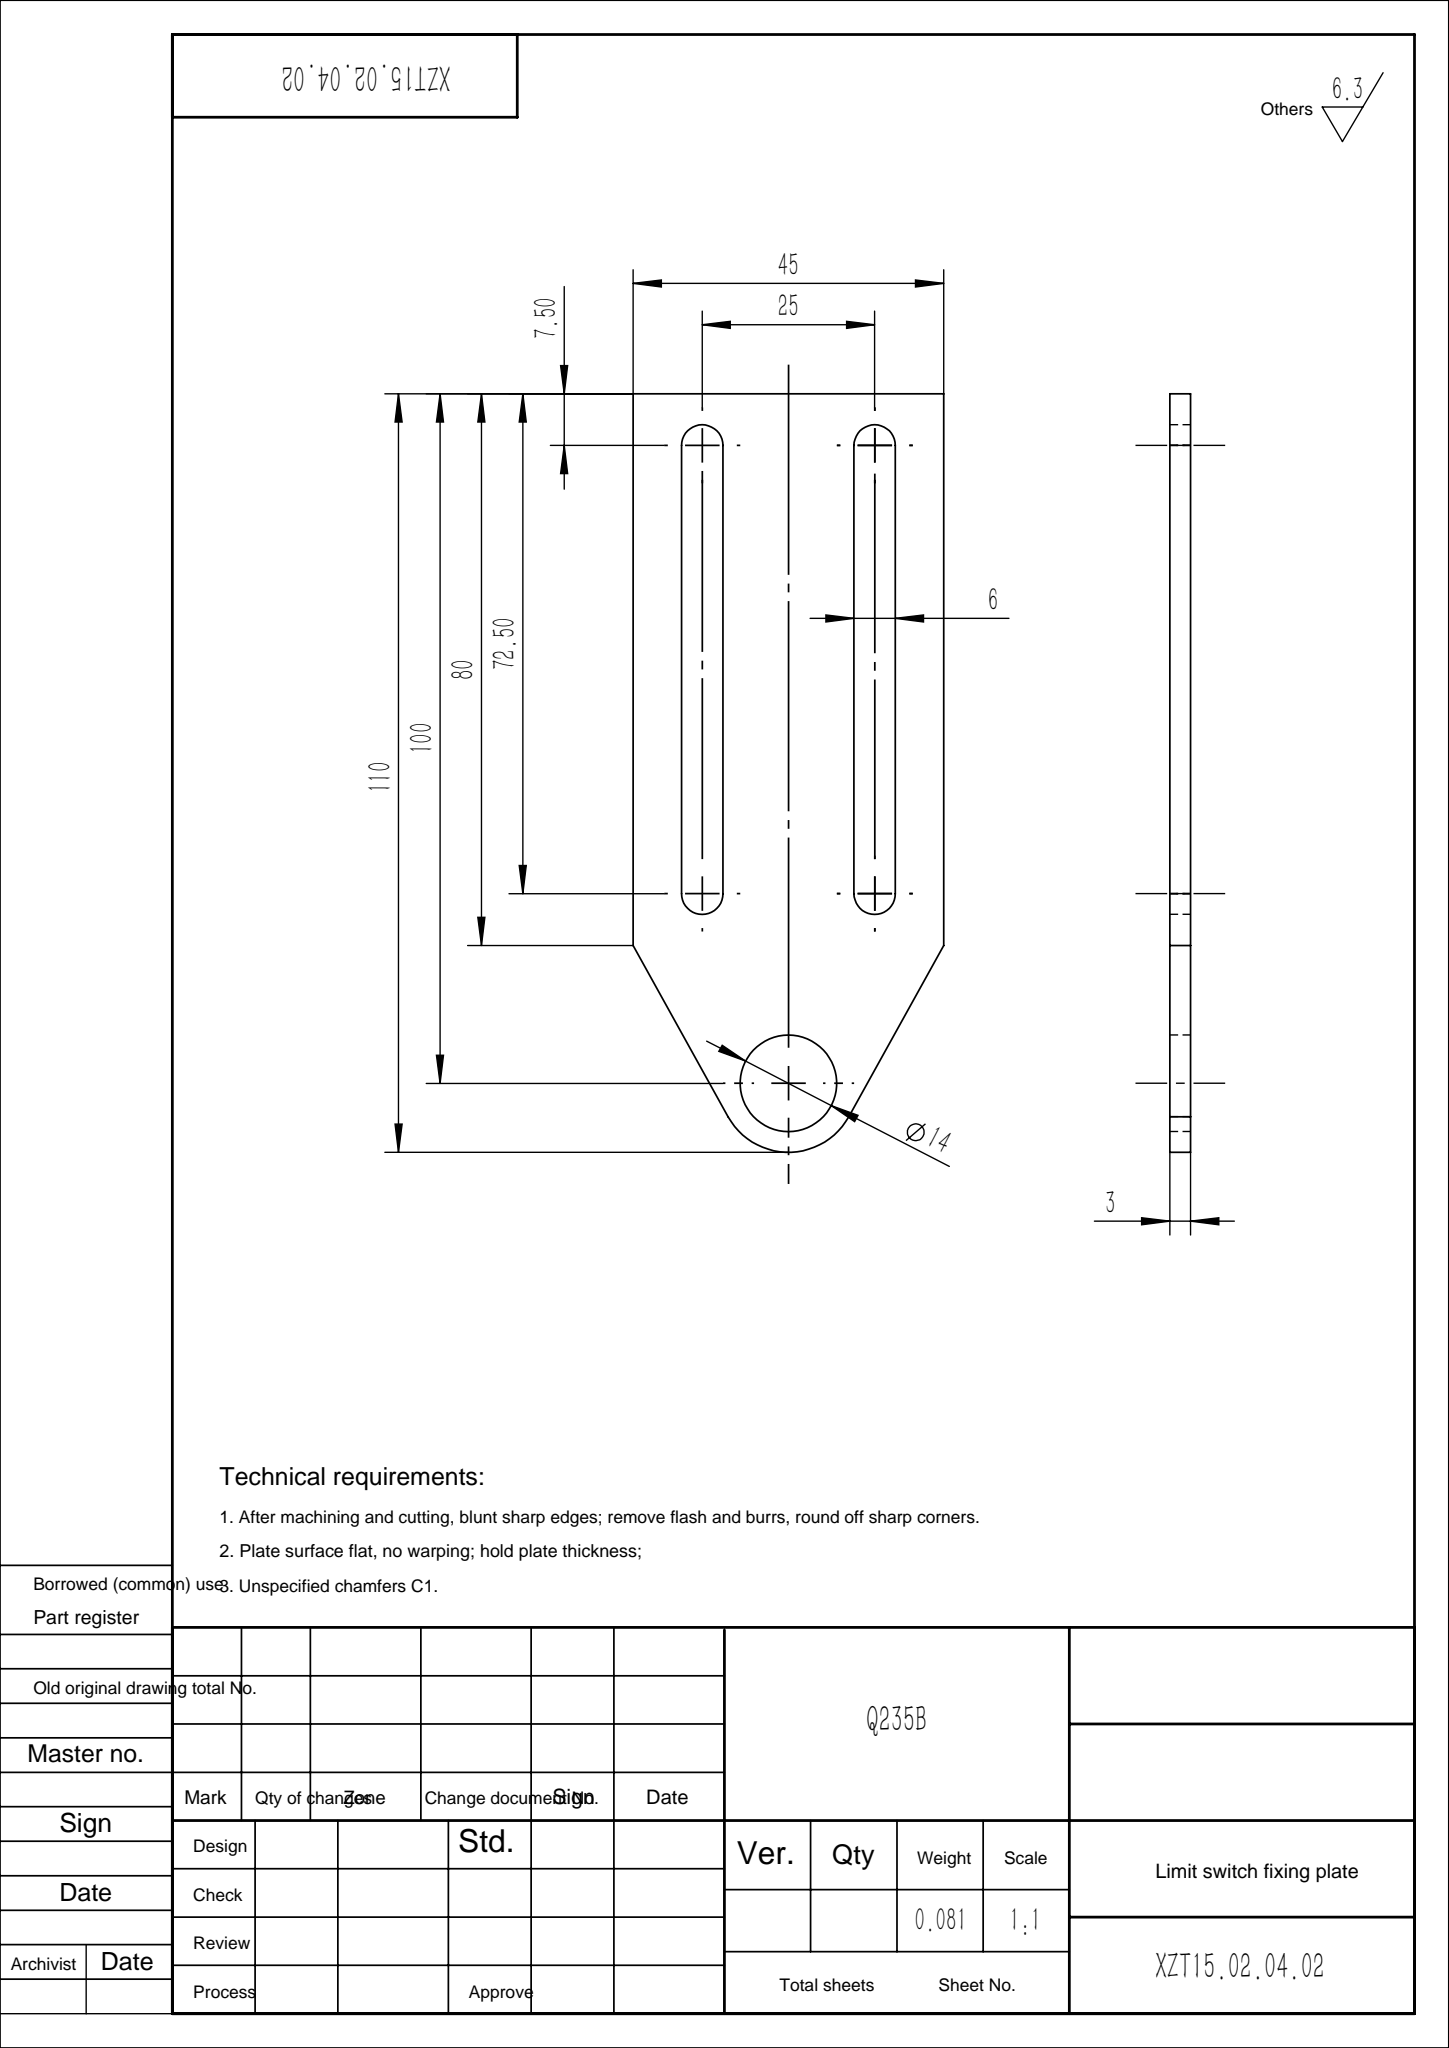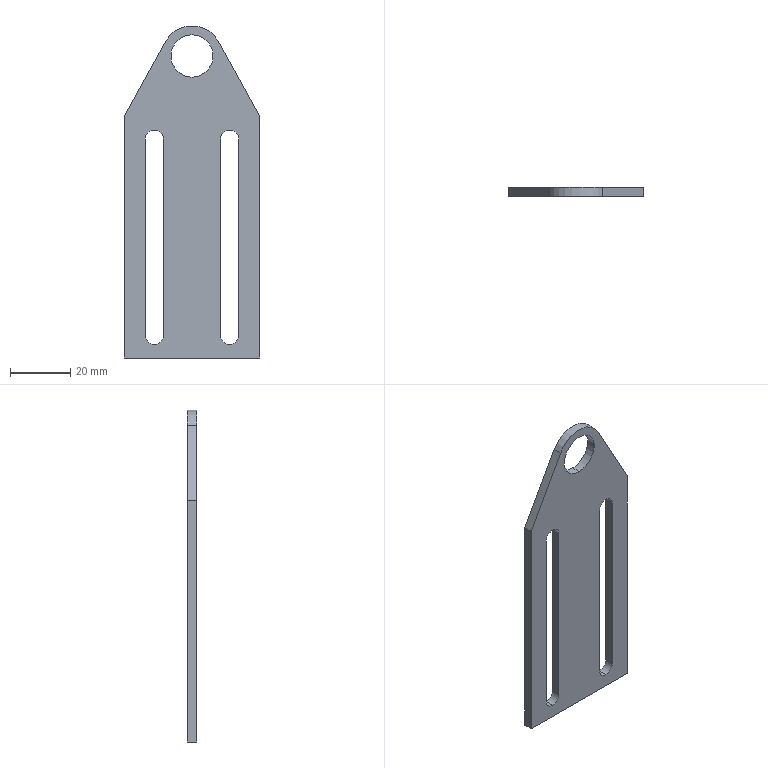Part | SolidWorks | features Extrusion 1 | 1 solid | 20 faces | box 45 x 3 x 110 mm | volume 10350 mm3 | plane 11 | cylinder 9 | commonest cylinder face diameters 6 x6 14 x2 20 x1
STEP:
#1=CARTESIAN_POINT('',(15.5,3.,-92.5));
#2=VERTEX_POINT('',#1);
#3=CARTESIAN_POINT('',(12.5,3.,-95.5));
#4=VERTEX_POINT('',#3);
#5=CARTESIAN_POINT('',(12.5,3.,-92.5));
#6=DIRECTION('',(0.,1.,0.));
#7=DIRECTION('',(0.,0.,-1.));
#8=AXIS2_PLACEMENT_3D('',#5,#6,#7);
#9=CIRCLE('',#8,3.);
#10=EDGE_CURVE('',#2,#4,#9,.T.);
#11=ORIENTED_EDGE('',*,*,#10,.T.);
#12=CARTESIAN_POINT('',(12.5,0.,-95.5));
#13=VERTEX_POINT('',#12);
#14=CARTESIAN_POINT('',(12.5,3.,-95.5));
#15=DIRECTION('',(0.,-1.,0.));
#16=VECTOR('',#15,1000.);
#17=LINE('',#14,#16);
#18=EDGE_CURVE('',#4,#13,#17,.T.);
#19=ORIENTED_EDGE('',*,*,#18,.T.);
#20=CARTESIAN_POINT('',(15.5,0.,-92.5));
#21=VERTEX_POINT('',#20);
#22=CARTESIAN_POINT('',(12.5,0.,-92.5));
#23=DIRECTION('',(0.,1.,0.));
#24=DIRECTION('',(0.,0.,-1.));
#25=AXIS2_PLACEMENT_3D('',#22,#23,#24);
#26=CIRCLE('',#25,3.);
#27=EDGE_CURVE('',#21,#13,#26,.T.);
#28=ORIENTED_EDGE('',*,*,#27,.F.);
#29=CARTESIAN_POINT('',(15.5,3.,-92.5));
#30=DIRECTION('',(0.,-1.,0.));
#31=VECTOR('',#30,1000.);
#32=LINE('',#29,#31);
#33=EDGE_CURVE('',#2,#21,#32,.T.);
#34=ORIENTED_EDGE('',*,*,#33,.F.);
#35=EDGE_LOOP('',(#11,#19,#28,#34));
#36=FACE_OUTER_BOUND('',#35,.T.);
#37=CARTESIAN_POINT('',(12.5,3.,-92.5));
#38=DIRECTION('',(0.,-1.,0.));
#39=DIRECTION('',(0.,0.,-1.));
#40=AXIS2_PLACEMENT_3D('',#37,#38,#39);
#41=CYLINDRICAL_SURFACE('',#40,3.);
#42=ADVANCED_FACE('',(#36),#41,.F.);
#43=CARTESIAN_POINT('',(0.,3.,-7.));
#44=VERTEX_POINT('',#43);
#45=CARTESIAN_POINT('',(0.,3.,7.));
#46=VERTEX_POINT('',#45);
#47=CARTESIAN_POINT('',(0.,3.,0.));
#48=DIRECTION('',(0.,1.,0.));
#49=DIRECTION('',(0.,0.,1.));
#50=AXIS2_PLACEMENT_3D('',#47,#48,#49);
#51=CIRCLE('',#50,7.);
#52=EDGE_CURVE('',#44,#46,#51,.T.);
#53=ORIENTED_EDGE('',*,*,#52,.T.);
#54=CARTESIAN_POINT('',(0.,0.,7.));
#55=VERTEX_POINT('',#54);
#56=CARTESIAN_POINT('',(0.,3.,7.));
#57=DIRECTION('',(0.,-1.,0.));
#58=VECTOR('',#57,1000.);
#59=LINE('',#56,#58);
#60=EDGE_CURVE('',#46,#55,#59,.T.);
#61=ORIENTED_EDGE('',*,*,#60,.T.);
#62=CARTESIAN_POINT('',(0.,0.,-7.));
#63=VERTEX_POINT('',#62);
#64=CARTESIAN_POINT('',(0.,0.,0.));
#65=DIRECTION('',(0.,1.,0.));
#66=DIRECTION('',(0.,0.,1.));
#67=AXIS2_PLACEMENT_3D('',#64,#65,#66);
#68=CIRCLE('',#67,7.);
#69=EDGE_CURVE('',#63,#55,#68,.T.);
#70=ORIENTED_EDGE('',*,*,#69,.F.);
#71=CARTESIAN_POINT('',(0.,3.,-7.));
#72=DIRECTION('',(0.,-1.,0.));
#73=VECTOR('',#72,1000.);
#74=LINE('',#71,#73);
#75=EDGE_CURVE('',#44,#63,#74,.T.);
#76=ORIENTED_EDGE('',*,*,#75,.F.);
#77=EDGE_LOOP('',(#53,#61,#70,#76));
#78=FACE_OUTER_BOUND('',#77,.T.);
#79=CARTESIAN_POINT('',(0.,3.,0.));
#80=DIRECTION('',(0.,-1.,0.));
#81=DIRECTION('',(0.,0.,-1.));
#82=AXIS2_PLACEMENT_3D('',#79,#80,#81);
#83=CYLINDRICAL_SURFACE('',#82,7.);
#84=ADVANCED_FACE('',(#78),#83,.F.);
#85=CARTESIAN_POINT('',(-9.5,3.,-92.5));
#86=VERTEX_POINT('',#85);
#87=CARTESIAN_POINT('',(-12.5,3.,-95.5));
#88=VERTEX_POINT('',#87);
#89=CARTESIAN_POINT('',(-12.5,3.,-92.5));
#90=DIRECTION('',(0.,1.,0.));
#91=DIRECTION('',(0.,0.,1.));
#92=AXIS2_PLACEMENT_3D('',#89,#90,#91);
#93=CIRCLE('',#92,3.);
#94=EDGE_CURVE('',#86,#88,#93,.T.);
#95=ORIENTED_EDGE('',*,*,#94,.T.);
#96=CARTESIAN_POINT('',(-12.5,0.,-95.5));
#97=VERTEX_POINT('',#96);
#98=CARTESIAN_POINT('',(-12.5,3.,-95.5));
#99=DIRECTION('',(0.,-1.,0.));
#100=VECTOR('',#99,1000.);
#101=LINE('',#98,#100);
#102=EDGE_CURVE('',#88,#97,#101,.T.);
#103=ORIENTED_EDGE('',*,*,#102,.T.);
#104=CARTESIAN_POINT('',(-9.5,0.,-92.5));
#105=VERTEX_POINT('',#104);
#106=CARTESIAN_POINT('',(-12.5,0.,-92.5));
#107=DIRECTION('',(0.,1.,0.));
#108=DIRECTION('',(0.,0.,1.));
#109=AXIS2_PLACEMENT_3D('',#106,#107,#108);
#110=CIRCLE('',#109,3.);
#111=EDGE_CURVE('',#105,#97,#110,.T.);
#112=ORIENTED_EDGE('',*,*,#111,.F.);
#113=CARTESIAN_POINT('',(-9.5,3.,-92.5));
#114=DIRECTION('',(0.,-1.,0.));
#115=VECTOR('',#114,1000.);
#116=LINE('',#113,#115);
#117=EDGE_CURVE('',#86,#105,#116,.T.);
#118=ORIENTED_EDGE('',*,*,#117,.F.);
#119=EDGE_LOOP('',(#95,#103,#112,#118));
#120=FACE_OUTER_BOUND('',#119,.T.);
#121=CARTESIAN_POINT('',(-12.5,3.,-92.5));
#122=DIRECTION('',(0.,-1.,0.));
#123=DIRECTION('',(0.,0.,-1.));
#124=AXIS2_PLACEMENT_3D('',#121,#122,#123);
#125=CYLINDRICAL_SURFACE('',#124,3.);
#126=ADVANCED_FACE('',(#120),#125,.F.);
#127=ORIENTED_EDGE('',*,*,#52,.F.);
#128=CARTESIAN_POINT('',(0.,3.,0.));
#129=DIRECTION('',(0.,1.,0.));
#130=DIRECTION('',(0.,0.,1.));
#131=AXIS2_PLACEMENT_3D('',#128,#129,#130);
#132=CIRCLE('',#131,7.);
#133=EDGE_CURVE('',#46,#44,#132,.T.);
#134=ORIENTED_EDGE('',*,*,#133,.F.);
#135=EDGE_LOOP('',(#127,#134));
#136=FACE_BOUND('',#135,.T.);
#137=CARTESIAN_POINT('',(-15.5,3.,-27.5));
#138=VERTEX_POINT('',#137);
#139=CARTESIAN_POINT('',(-9.5,3.,-27.5));
#140=VERTEX_POINT('',#139);
#141=CARTESIAN_POINT('',(-12.5,3.,-27.5));
#142=DIRECTION('',(0.,1.,0.));
#143=DIRECTION('',(0.,0.,1.));
#144=AXIS2_PLACEMENT_3D('',#141,#142,#143);
#145=CIRCLE('',#144,3.);
#146=EDGE_CURVE('',#138,#140,#145,.T.);
#147=ORIENTED_EDGE('',*,*,#146,.F.);
#148=CARTESIAN_POINT('',(-15.5,3.,-92.5));
#149=VERTEX_POINT('',#148);
#150=CARTESIAN_POINT('',(-15.5,3.,-27.5));
#151=DIRECTION('',(0.,0.,1.));
#152=VECTOR('',#151,1000.);
#153=LINE('',#150,#152);
#154=EDGE_CURVE('',#149,#138,#153,.T.);
#155=ORIENTED_EDGE('',*,*,#154,.F.);
#156=CARTESIAN_POINT('',(-12.5,3.,-92.5));
#157=DIRECTION('',(0.,1.,0.));
#158=DIRECTION('',(0.,0.,1.));
#159=AXIS2_PLACEMENT_3D('',#156,#157,#158);
#160=CIRCLE('',#159,3.);
#161=EDGE_CURVE('',#88,#149,#160,.T.);
#162=ORIENTED_EDGE('',*,*,#161,.F.);
#163=ORIENTED_EDGE('',*,*,#94,.F.);
#164=CARTESIAN_POINT('',(-9.5,3.,-27.5));
#165=DIRECTION('',(0.,0.,-1.));
#166=VECTOR('',#165,1000.);
#167=LINE('',#164,#166);
#168=EDGE_CURVE('',#140,#86,#167,.T.);
#169=ORIENTED_EDGE('',*,*,#168,.F.);
#170=EDGE_LOOP('',(#147,#155,#162,#163,#169));
#171=FACE_BOUND('',#170,.T.);
#172=CARTESIAN_POINT('',(22.5,3.,-20.));
#173=VERTEX_POINT('',#172);
#174=CARTESIAN_POINT('',(22.5,3.,-100.));
#175=VERTEX_POINT('',#174);
#176=CARTESIAN_POINT('',(22.5,3.,-100.));
#177=DIRECTION('',(0.,0.,-1.));
#178=VECTOR('',#177,1000.);
#179=LINE('',#176,#178);
#180=EDGE_CURVE('',#173,#175,#179,.T.);
#181=ORIENTED_EDGE('',*,*,#180,.T.);
#182=CARTESIAN_POINT('',(-22.5,3.,-100.));
#183=VERTEX_POINT('',#182);
#184=CARTESIAN_POINT('',(-22.5,3.,-100.));
#185=DIRECTION('',(-1.,0.,0.));
#186=VECTOR('',#185,1000.);
#187=LINE('',#184,#186);
#188=EDGE_CURVE('',#175,#183,#187,.T.);
#189=ORIENTED_EDGE('',*,*,#188,.T.);
#190=CARTESIAN_POINT('',(-22.5,3.,-20.));
#191=VERTEX_POINT('',#190);
#192=CARTESIAN_POINT('',(-22.5,3.,-100.));
#193=DIRECTION('',(0.,0.,1.));
#194=VECTOR('',#193,1000.);
#195=LINE('',#192,#194);
#196=EDGE_CURVE('',#183,#191,#195,.T.);
#197=ORIENTED_EDGE('',*,*,#196,.T.);
#198=CARTESIAN_POINT('',(-8.749,3.,4.843));
#199=VERTEX_POINT('',#198);
#200=CARTESIAN_POINT('',(-22.5,3.,-20.));
#201=DIRECTION('',(0.4843,0.,0.8749));
#202=VECTOR('',#201,1000.);
#203=LINE('',#200,#202);
#204=EDGE_CURVE('',#191,#199,#203,.T.);
#205=ORIENTED_EDGE('',*,*,#204,.T.);
#206=CARTESIAN_POINT('',(8.749,3.,4.843));
#207=VERTEX_POINT('',#206);
#208=CARTESIAN_POINT('',(0.,3.,0.));
#209=DIRECTION('',(0.,1.,0.));
#210=DIRECTION('',(0.,0.,-1.));
#211=AXIS2_PLACEMENT_3D('',#208,#209,#210);
#212=CIRCLE('',#211,10.);
#213=EDGE_CURVE('',#199,#207,#212,.T.);
#214=ORIENTED_EDGE('',*,*,#213,.T.);
#215=CARTESIAN_POINT('',(22.5,3.,-20.));
#216=DIRECTION('',(0.4843,0.,-0.8749));
#217=VECTOR('',#216,1000.);
#218=LINE('',#215,#217);
#219=EDGE_CURVE('',#207,#173,#218,.T.);
#220=ORIENTED_EDGE('',*,*,#219,.T.);
#221=EDGE_LOOP('',(#181,#189,#197,#205,#214,#220));
#222=FACE_OUTER_BOUND('',#221,.T.);
#223=CARTESIAN_POINT('',(9.5,3.,-27.5));
#224=VERTEX_POINT('',#223);
#225=CARTESIAN_POINT('',(15.5,3.,-27.5));
#226=VERTEX_POINT('',#225);
#227=CARTESIAN_POINT('',(12.5,3.,-27.5));
#228=DIRECTION('',(0.,1.,0.));
#229=DIRECTION('',(0.,0.,-1.));
#230=AXIS2_PLACEMENT_3D('',#227,#228,#229);
#231=CIRCLE('',#230,3.);
#232=EDGE_CURVE('',#224,#226,#231,.T.);
#233=ORIENTED_EDGE('',*,*,#232,.F.);
#234=CARTESIAN_POINT('',(9.5,3.,-92.5));
#235=VERTEX_POINT('',#234);
#236=CARTESIAN_POINT('',(9.5,3.,-27.5));
#237=DIRECTION('',(0.,0.,1.));
#238=VECTOR('',#237,1000.);
#239=LINE('',#236,#238);
#240=EDGE_CURVE('',#235,#224,#239,.T.);
#241=ORIENTED_EDGE('',*,*,#240,.F.);
#242=CARTESIAN_POINT('',(12.5,3.,-92.5));
#243=DIRECTION('',(0.,1.,0.));
#244=DIRECTION('',(0.,0.,-1.));
#245=AXIS2_PLACEMENT_3D('',#242,#243,#244);
#246=CIRCLE('',#245,3.);
#247=EDGE_CURVE('',#4,#235,#246,.T.);
#248=ORIENTED_EDGE('',*,*,#247,.F.);
#249=ORIENTED_EDGE('',*,*,#10,.F.);
#250=CARTESIAN_POINT('',(15.5,3.,-27.5));
#251=DIRECTION('',(0.,0.,-1.));
#252=VECTOR('',#251,1000.);
#253=LINE('',#250,#252);
#254=EDGE_CURVE('',#226,#2,#253,.T.);
#255=ORIENTED_EDGE('',*,*,#254,.F.);
#256=EDGE_LOOP('',(#233,#241,#248,#249,#255));
#257=FACE_BOUND('',#256,.T.);
#258=CARTESIAN_POINT('',(0.,3.,0.));
#259=DIRECTION('',(0.,-1.,0.));
#260=DIRECTION('',(0.,0.,-1.));
#261=AXIS2_PLACEMENT_3D('',#258,#259,#260);
#262=PLANE('',#261);
#263=ADVANCED_FACE('',(#136,#171,#222,#257),#262,.F.);
#264=CARTESIAN_POINT('',(-15.5,0.,-92.5));
#265=VERTEX_POINT('',#264);
#266=CARTESIAN_POINT('',(-15.5,0.,-27.5));
#267=VERTEX_POINT('',#266);
#268=CARTESIAN_POINT('',(-15.5,0.,-27.5));
#269=DIRECTION('',(0.,0.,1.));
#270=VECTOR('',#269,1000.);
#271=LINE('',#268,#270);
#272=EDGE_CURVE('',#265,#267,#271,.T.);
#273=ORIENTED_EDGE('',*,*,#272,.T.);
#274=CARTESIAN_POINT('',(-9.5,0.,-27.5));
#275=VERTEX_POINT('',#274);
#276=CARTESIAN_POINT('',(-12.5,0.,-27.5));
#277=DIRECTION('',(0.,1.,0.));
#278=DIRECTION('',(0.,0.,1.));
#279=AXIS2_PLACEMENT_3D('',#276,#277,#278);
#280=CIRCLE('',#279,3.);
#281=EDGE_CURVE('',#267,#275,#280,.T.);
#282=ORIENTED_EDGE('',*,*,#281,.T.);
#283=CARTESIAN_POINT('',(-9.5,0.,-27.5));
#284=DIRECTION('',(0.,0.,-1.));
#285=VECTOR('',#284,1000.);
#286=LINE('',#283,#285);
#287=EDGE_CURVE('',#275,#105,#286,.T.);
#288=ORIENTED_EDGE('',*,*,#287,.T.);
#289=ORIENTED_EDGE('',*,*,#111,.T.);
#290=CARTESIAN_POINT('',(-12.5,0.,-92.5));
#291=DIRECTION('',(0.,1.,0.));
#292=DIRECTION('',(0.,0.,1.));
#293=AXIS2_PLACEMENT_3D('',#290,#291,#292);
#294=CIRCLE('',#293,3.);
#295=EDGE_CURVE('',#97,#265,#294,.T.);
#296=ORIENTED_EDGE('',*,*,#295,.T.);
#297=EDGE_LOOP('',(#273,#282,#288,#289,#296));
#298=FACE_BOUND('',#297,.T.);
#299=CARTESIAN_POINT('',(22.5,0.,-20.));
#300=VERTEX_POINT('',#299);
#301=CARTESIAN_POINT('',(22.5,0.,-100.));
#302=VERTEX_POINT('',#301);
#303=CARTESIAN_POINT('',(22.5,0.,-100.));
#304=DIRECTION('',(0.,0.,-1.));
#305=VECTOR('',#304,1000.);
#306=LINE('',#303,#305);
#307=EDGE_CURVE('',#300,#302,#306,.T.);
#308=ORIENTED_EDGE('',*,*,#307,.F.);
#309=CARTESIAN_POINT('',(8.749,0.,4.843));
#310=VERTEX_POINT('',#309);
#311=CARTESIAN_POINT('',(22.5,0.,-20.));
#312=DIRECTION('',(0.4843,0.,-0.8749));
#313=VECTOR('',#312,1000.);
#314=LINE('',#311,#313);
#315=EDGE_CURVE('',#310,#300,#314,.T.);
#316=ORIENTED_EDGE('',*,*,#315,.F.);
#317=CARTESIAN_POINT('',(-8.749,0.,4.843));
#318=VERTEX_POINT('',#317);
#319=CARTESIAN_POINT('',(0.,0.,0.));
#320=DIRECTION('',(0.,1.,0.));
#321=DIRECTION('',(0.,0.,-1.));
#322=AXIS2_PLACEMENT_3D('',#319,#320,#321);
#323=CIRCLE('',#322,10.);
#324=EDGE_CURVE('',#318,#310,#323,.T.);
#325=ORIENTED_EDGE('',*,*,#324,.F.);
#326=CARTESIAN_POINT('',(-22.5,0.,-20.));
#327=VERTEX_POINT('',#326);
#328=CARTESIAN_POINT('',(-22.5,0.,-20.));
#329=DIRECTION('',(0.4843,0.,0.8749));
#330=VECTOR('',#329,1000.);
#331=LINE('',#328,#330);
#332=EDGE_CURVE('',#327,#318,#331,.T.);
#333=ORIENTED_EDGE('',*,*,#332,.F.);
#334=CARTESIAN_POINT('',(-22.5,0.,-100.));
#335=VERTEX_POINT('',#334);
#336=CARTESIAN_POINT('',(-22.5,0.,-100.));
#337=DIRECTION('',(0.,0.,1.));
#338=VECTOR('',#337,1000.);
#339=LINE('',#336,#338);
#340=EDGE_CURVE('',#335,#327,#339,.T.);
#341=ORIENTED_EDGE('',*,*,#340,.F.);
#342=CARTESIAN_POINT('',(-22.5,0.,-100.));
#343=DIRECTION('',(-1.,0.,0.));
#344=VECTOR('',#343,1000.);
#345=LINE('',#342,#344);
#346=EDGE_CURVE('',#302,#335,#345,.T.);
#347=ORIENTED_EDGE('',*,*,#346,.F.);
#348=EDGE_LOOP('',(#308,#316,#325,#333,#341,#347));
#349=FACE_OUTER_BOUND('',#348,.T.);
#350=ORIENTED_EDGE('',*,*,#69,.T.);
#351=CARTESIAN_POINT('',(0.,0.,0.));
#352=DIRECTION('',(0.,1.,0.));
#353=DIRECTION('',(0.,0.,1.));
#354=AXIS2_PLACEMENT_3D('',#351,#352,#353);
#355=CIRCLE('',#354,7.);
#356=EDGE_CURVE('',#55,#63,#355,.T.);
#357=ORIENTED_EDGE('',*,*,#356,.T.);
#358=EDGE_LOOP('',(#350,#357));
#359=FACE_BOUND('',#358,.T.);
#360=CARTESIAN_POINT('',(9.5,0.,-92.5));
#361=VERTEX_POINT('',#360);
#362=CARTESIAN_POINT('',(9.5,0.,-27.5));
#363=VERTEX_POINT('',#362);
#364=CARTESIAN_POINT('',(9.5,0.,-27.5));
#365=DIRECTION('',(0.,0.,1.));
#366=VECTOR('',#365,1000.);
#367=LINE('',#364,#366);
#368=EDGE_CURVE('',#361,#363,#367,.T.);
#369=ORIENTED_EDGE('',*,*,#368,.T.);
#370=CARTESIAN_POINT('',(15.5,0.,-27.5));
#371=VERTEX_POINT('',#370);
#372=CARTESIAN_POINT('',(12.5,0.,-27.5));
#373=DIRECTION('',(0.,1.,0.));
#374=DIRECTION('',(0.,0.,-1.));
#375=AXIS2_PLACEMENT_3D('',#372,#373,#374);
#376=CIRCLE('',#375,3.);
#377=EDGE_CURVE('',#363,#371,#376,.T.);
#378=ORIENTED_EDGE('',*,*,#377,.T.);
#379=CARTESIAN_POINT('',(15.5,0.,-27.5));
#380=DIRECTION('',(0.,0.,-1.));
#381=VECTOR('',#380,1000.);
#382=LINE('',#379,#381);
#383=EDGE_CURVE('',#371,#21,#382,.T.);
#384=ORIENTED_EDGE('',*,*,#383,.T.);
#385=ORIENTED_EDGE('',*,*,#27,.T.);
#386=CARTESIAN_POINT('',(12.5,0.,-92.5));
#387=DIRECTION('',(0.,1.,0.));
#388=DIRECTION('',(0.,0.,-1.));
#389=AXIS2_PLACEMENT_3D('',#386,#387,#388);
#390=CIRCLE('',#389,3.);
#391=EDGE_CURVE('',#13,#361,#390,.T.);
#392=ORIENTED_EDGE('',*,*,#391,.T.);
#393=EDGE_LOOP('',(#369,#378,#384,#385,#392));
#394=FACE_BOUND('',#393,.T.);
#395=CARTESIAN_POINT('',(0.,0.,0.));
#396=DIRECTION('',(0.,-1.,0.));
#397=DIRECTION('',(0.,0.,-1.));
#398=AXIS2_PLACEMENT_3D('',#395,#396,#397);
#399=PLANE('',#398);
#400=ADVANCED_FACE('',(#298,#349,#359,#394),#399,.T.);
#401=ORIENTED_EDGE('',*,*,#307,.T.);
#402=CARTESIAN_POINT('',(22.5,3.,-100.));
#403=DIRECTION('',(0.,-1.,0.));
#404=VECTOR('',#403,1000.);
#405=LINE('',#402,#404);
#406=EDGE_CURVE('',#175,#302,#405,.T.);
#407=ORIENTED_EDGE('',*,*,#406,.F.);
#408=ORIENTED_EDGE('',*,*,#180,.F.);
#409=CARTESIAN_POINT('',(22.5,3.,-20.));
#410=DIRECTION('',(0.,-1.,0.));
#411=VECTOR('',#410,1000.);
#412=LINE('',#409,#411);
#413=EDGE_CURVE('',#173,#300,#412,.T.);
#414=ORIENTED_EDGE('',*,*,#413,.T.);
#415=EDGE_LOOP('',(#401,#407,#408,#414));
#416=FACE_OUTER_BOUND('',#415,.T.);
#417=CARTESIAN_POINT('',(22.5,3.,-100.));
#418=DIRECTION('',(-1.,0.,0.));
#419=DIRECTION('',(0.,0.,1.));
#420=AXIS2_PLACEMENT_3D('',#417,#418,#419);
#421=PLANE('',#420);
#422=ADVANCED_FACE('',(#416),#421,.F.);
#423=ORIENTED_EDGE('',*,*,#346,.T.);
#424=CARTESIAN_POINT('',(-22.5,3.,-100.));
#425=DIRECTION('',(0.,-1.,0.));
#426=VECTOR('',#425,1000.);
#427=LINE('',#424,#426);
#428=EDGE_CURVE('',#183,#335,#427,.T.);
#429=ORIENTED_EDGE('',*,*,#428,.F.);
#430=ORIENTED_EDGE('',*,*,#188,.F.);
#431=ORIENTED_EDGE('',*,*,#406,.T.);
#432=EDGE_LOOP('',(#423,#429,#430,#431));
#433=FACE_OUTER_BOUND('',#432,.T.);
#434=CARTESIAN_POINT('',(-22.5,3.,-100.));
#435=DIRECTION('',(0.,0.,1.));
#436=DIRECTION('',(1.,0.,0.));
#437=AXIS2_PLACEMENT_3D('',#434,#435,#436);
#438=PLANE('',#437);
#439=ADVANCED_FACE('',(#433),#438,.F.);
#440=ORIENTED_EDGE('',*,*,#340,.T.);
#441=CARTESIAN_POINT('',(-22.5,3.,-20.));
#442=DIRECTION('',(0.,-1.,0.));
#443=VECTOR('',#442,1000.);
#444=LINE('',#441,#443);
#445=EDGE_CURVE('',#191,#327,#444,.T.);
#446=ORIENTED_EDGE('',*,*,#445,.F.);
#447=ORIENTED_EDGE('',*,*,#196,.F.);
#448=ORIENTED_EDGE('',*,*,#428,.T.);
#449=EDGE_LOOP('',(#440,#446,#447,#448));
#450=FACE_OUTER_BOUND('',#449,.T.);
#451=CARTESIAN_POINT('',(-22.5,3.,-100.));
#452=DIRECTION('',(1.,0.,0.));
#453=DIRECTION('',(0.,0.,-1.));
#454=AXIS2_PLACEMENT_3D('',#451,#452,#453);
#455=PLANE('',#454);
#456=ADVANCED_FACE('',(#450),#455,.F.);
#457=ORIENTED_EDGE('',*,*,#332,.T.);
#458=CARTESIAN_POINT('',(-8.749,3.,4.843));
#459=DIRECTION('',(0.,-1.,0.));
#460=VECTOR('',#459,1000.);
#461=LINE('',#458,#460);
#462=EDGE_CURVE('',#199,#318,#461,.T.);
#463=ORIENTED_EDGE('',*,*,#462,.F.);
#464=ORIENTED_EDGE('',*,*,#204,.F.);
#465=ORIENTED_EDGE('',*,*,#445,.T.);
#466=EDGE_LOOP('',(#457,#463,#464,#465));
#467=FACE_OUTER_BOUND('',#466,.T.);
#468=CARTESIAN_POINT('',(-22.5,3.,-20.));
#469=DIRECTION('',(0.8749,0.,-0.4843));
#470=DIRECTION('',(-0.4843,0.,-0.8749));
#471=AXIS2_PLACEMENT_3D('',#468,#469,#470);
#472=PLANE('',#471);
#473=ADVANCED_FACE('',(#467),#472,.F.);
#474=ORIENTED_EDGE('',*,*,#324,.T.);
#475=CARTESIAN_POINT('',(8.749,3.,4.843));
#476=DIRECTION('',(0.,-1.,0.));
#477=VECTOR('',#476,1000.);
#478=LINE('',#475,#477);
#479=EDGE_CURVE('',#207,#310,#478,.T.);
#480=ORIENTED_EDGE('',*,*,#479,.F.);
#481=ORIENTED_EDGE('',*,*,#213,.F.);
#482=ORIENTED_EDGE('',*,*,#462,.T.);
#483=EDGE_LOOP('',(#474,#480,#481,#482));
#484=FACE_OUTER_BOUND('',#483,.T.);
#485=CARTESIAN_POINT('',(0.,3.,0.));
#486=DIRECTION('',(0.,-1.,0.));
#487=DIRECTION('',(0.,0.,-1.));
#488=AXIS2_PLACEMENT_3D('',#485,#486,#487);
#489=CYLINDRICAL_SURFACE('',#488,10.);
#490=ADVANCED_FACE('',(#484),#489,.T.);
#491=ORIENTED_EDGE('',*,*,#315,.T.);
#492=ORIENTED_EDGE('',*,*,#413,.F.);
#493=ORIENTED_EDGE('',*,*,#219,.F.);
#494=ORIENTED_EDGE('',*,*,#479,.T.);
#495=EDGE_LOOP('',(#491,#492,#493,#494));
#496=FACE_OUTER_BOUND('',#495,.T.);
#497=CARTESIAN_POINT('',(22.5,3.,-20.));
#498=DIRECTION('',(-0.8749,0.,-0.4843));
#499=DIRECTION('',(-0.4843,0.,0.8749));
#500=AXIS2_PLACEMENT_3D('',#497,#498,#499);
#501=PLANE('',#500);
#502=ADVANCED_FACE('',(#496),#501,.F.);
#503=ORIENTED_EDGE('',*,*,#281,.F.);
#504=CARTESIAN_POINT('',(-15.5,3.,-27.5));
#505=DIRECTION('',(0.,-1.,0.));
#506=VECTOR('',#505,1000.);
#507=LINE('',#504,#506);
#508=EDGE_CURVE('',#138,#267,#507,.T.);
#509=ORIENTED_EDGE('',*,*,#508,.F.);
#510=ORIENTED_EDGE('',*,*,#146,.T.);
#511=CARTESIAN_POINT('',(-9.5,3.,-27.5));
#512=DIRECTION('',(0.,-1.,0.));
#513=VECTOR('',#512,1000.);
#514=LINE('',#511,#513);
#515=EDGE_CURVE('',#140,#275,#514,.T.);
#516=ORIENTED_EDGE('',*,*,#515,.T.);
#517=EDGE_LOOP('',(#503,#509,#510,#516));
#518=FACE_OUTER_BOUND('',#517,.T.);
#519=CARTESIAN_POINT('',(-12.5,3.,-27.5));
#520=DIRECTION('',(0.,-1.,0.));
#521=DIRECTION('',(0.,0.,-1.));
#522=AXIS2_PLACEMENT_3D('',#519,#520,#521);
#523=CYLINDRICAL_SURFACE('',#522,3.);
#524=ADVANCED_FACE('',(#518),#523,.F.);
#525=ORIENTED_EDGE('',*,*,#287,.F.);
#526=ORIENTED_EDGE('',*,*,#515,.F.);
#527=ORIENTED_EDGE('',*,*,#168,.T.);
#528=ORIENTED_EDGE('',*,*,#117,.T.);
#529=EDGE_LOOP('',(#525,#526,#527,#528));
#530=FACE_OUTER_BOUND('',#529,.T.);
#531=CARTESIAN_POINT('',(-9.5,3.,-27.5));
#532=DIRECTION('',(-1.,0.,0.));
#533=DIRECTION('',(0.,0.,1.));
#534=AXIS2_PLACEMENT_3D('',#531,#532,#533);
#535=PLANE('',#534);
#536=ADVANCED_FACE('',(#530),#535,.T.);
#537=ORIENTED_EDGE('',*,*,#102,.F.);
#538=ORIENTED_EDGE('',*,*,#161,.T.);
#539=CARTESIAN_POINT('',(-15.5,3.,-92.5));
#540=DIRECTION('',(0.,-1.,0.));
#541=VECTOR('',#540,1000.);
#542=LINE('',#539,#541);
#543=EDGE_CURVE('',#149,#265,#542,.T.);
#544=ORIENTED_EDGE('',*,*,#543,.T.);
#545=ORIENTED_EDGE('',*,*,#295,.F.);
#546=EDGE_LOOP('',(#537,#538,#544,#545));
#547=FACE_OUTER_BOUND('',#546,.T.);
#548=CARTESIAN_POINT('',(-12.5,3.,-92.5));
#549=DIRECTION('',(0.,-1.,0.));
#550=DIRECTION('',(0.,0.,-1.));
#551=AXIS2_PLACEMENT_3D('',#548,#549,#550);
#552=CYLINDRICAL_SURFACE('',#551,3.);
#553=ADVANCED_FACE('',(#547),#552,.F.);
#554=ORIENTED_EDGE('',*,*,#272,.F.);
#555=ORIENTED_EDGE('',*,*,#543,.F.);
#556=ORIENTED_EDGE('',*,*,#154,.T.);
#557=ORIENTED_EDGE('',*,*,#508,.T.);
#558=EDGE_LOOP('',(#554,#555,#556,#557));
#559=FACE_OUTER_BOUND('',#558,.T.);
#560=CARTESIAN_POINT('',(-15.5,3.,-27.5));
#561=DIRECTION('',(1.,0.,0.));
#562=DIRECTION('',(0.,0.,-1.));
#563=AXIS2_PLACEMENT_3D('',#560,#561,#562);
#564=PLANE('',#563);
#565=ADVANCED_FACE('',(#559),#564,.T.);
#566=ORIENTED_EDGE('',*,*,#60,.F.);
#567=ORIENTED_EDGE('',*,*,#133,.T.);
#568=ORIENTED_EDGE('',*,*,#75,.T.);
#569=ORIENTED_EDGE('',*,*,#356,.F.);
#570=EDGE_LOOP('',(#566,#567,#568,#569));
#571=FACE_OUTER_BOUND('',#570,.T.);
#572=CARTESIAN_POINT('',(0.,3.,0.));
#573=DIRECTION('',(0.,-1.,0.));
#574=DIRECTION('',(0.,0.,-1.));
#575=AXIS2_PLACEMENT_3D('',#572,#573,#574);
#576=CYLINDRICAL_SURFACE('',#575,7.);
#577=ADVANCED_FACE('',(#571),#576,.F.);
#578=ORIENTED_EDGE('',*,*,#377,.F.);
#579=CARTESIAN_POINT('',(9.5,3.,-27.5));
#580=DIRECTION('',(0.,-1.,0.));
#581=VECTOR('',#580,1000.);
#582=LINE('',#579,#581);
#583=EDGE_CURVE('',#224,#363,#582,.T.);
#584=ORIENTED_EDGE('',*,*,#583,.F.);
#585=ORIENTED_EDGE('',*,*,#232,.T.);
#586=CARTESIAN_POINT('',(15.5,3.,-27.5));
#587=DIRECTION('',(0.,-1.,0.));
#588=VECTOR('',#587,1000.);
#589=LINE('',#586,#588);
#590=EDGE_CURVE('',#226,#371,#589,.T.);
#591=ORIENTED_EDGE('',*,*,#590,.T.);
#592=EDGE_LOOP('',(#578,#584,#585,#591));
#593=FACE_OUTER_BOUND('',#592,.T.);
#594=CARTESIAN_POINT('',(12.5,3.,-27.5));
#595=DIRECTION('',(0.,-1.,0.));
#596=DIRECTION('',(0.,0.,-1.));
#597=AXIS2_PLACEMENT_3D('',#594,#595,#596);
#598=CYLINDRICAL_SURFACE('',#597,3.);
#599=ADVANCED_FACE('',(#593),#598,.F.);
#600=ORIENTED_EDGE('',*,*,#383,.F.);
#601=ORIENTED_EDGE('',*,*,#590,.F.);
#602=ORIENTED_EDGE('',*,*,#254,.T.);
#603=ORIENTED_EDGE('',*,*,#33,.T.);
#604=EDGE_LOOP('',(#600,#601,#602,#603));
#605=FACE_OUTER_BOUND('',#604,.T.);
#606=CARTESIAN_POINT('',(15.5,3.,-27.5));
#607=DIRECTION('',(-1.,0.,0.));
#608=DIRECTION('',(0.,0.,1.));
#609=AXIS2_PLACEMENT_3D('',#606,#607,#608);
#610=PLANE('',#609);
#611=ADVANCED_FACE('',(#605),#610,.T.);
#612=ORIENTED_EDGE('',*,*,#18,.F.);
#613=ORIENTED_EDGE('',*,*,#247,.T.);
#614=CARTESIAN_POINT('',(9.5,3.,-92.5));
#615=DIRECTION('',(0.,-1.,0.));
#616=VECTOR('',#615,1000.);
#617=LINE('',#614,#616);
#618=EDGE_CURVE('',#235,#361,#617,.T.);
#619=ORIENTED_EDGE('',*,*,#618,.T.);
#620=ORIENTED_EDGE('',*,*,#391,.F.);
#621=EDGE_LOOP('',(#612,#613,#619,#620));
#622=FACE_OUTER_BOUND('',#621,.T.);
#623=CARTESIAN_POINT('',(12.5,3.,-92.5));
#624=DIRECTION('',(0.,-1.,0.));
#625=DIRECTION('',(0.,0.,-1.));
#626=AXIS2_PLACEMENT_3D('',#623,#624,#625);
#627=CYLINDRICAL_SURFACE('',#626,3.);
#628=ADVANCED_FACE('',(#622),#627,.F.);
#629=ORIENTED_EDGE('',*,*,#368,.F.);
#630=ORIENTED_EDGE('',*,*,#618,.F.);
#631=ORIENTED_EDGE('',*,*,#240,.T.);
#632=ORIENTED_EDGE('',*,*,#583,.T.);
#633=EDGE_LOOP('',(#629,#630,#631,#632));
#634=FACE_OUTER_BOUND('',#633,.T.);
#635=CARTESIAN_POINT('',(9.5,3.,-27.5));
#636=DIRECTION('',(1.,0.,0.));
#637=DIRECTION('',(0.,0.,-1.));
#638=AXIS2_PLACEMENT_3D('',#635,#636,#637);
#639=PLANE('',#638);
#640=ADVANCED_FACE('',(#634),#639,.T.);
#641=CLOSED_SHELL('',(#42,#84,#126,#263,#400,#422,#439,#456,#473,#490,#502,#524,#536,#553,#565,#577,#599,#611,#628,#640));
#642=MANIFOLD_SOLID_BREP('',#641);
#643=CARTESIAN_POINT('',(0.,0.,0.));
#644=DIRECTION('',(0.,0.,1.));
#645=DIRECTION('',(1.,0.,0.));
#646=AXIS2_PLACEMENT_3D('',#643,#644,#645);
#647=(LENGTH_UNIT()NAMED_UNIT(*)SI_UNIT(.MILLI.,.METRE.));
#648=UNCERTAINTY_MEASURE_WITH_UNIT(LENGTH_MEASURE(0.00001),#647,'','');
#649=(NAMED_UNIT(*)PLANE_ANGLE_UNIT()SI_UNIT($,.RADIAN.));
#650=(NAMED_UNIT(*)SI_UNIT($,.STERADIAN.)SOLID_ANGLE_UNIT());
#651=(GEOMETRIC_REPRESENTATION_CONTEXT(3)GLOBAL_UNCERTAINTY_ASSIGNED_CONTEXT((#648))GLOBAL_UNIT_ASSIGNED_CONTEXT((#647,#649,#650))REPRESENTATION_CONTEXT('',''));
#652=ADVANCED_BREP_SHAPE_REPRESENTATION('',(#642,#646),#651);